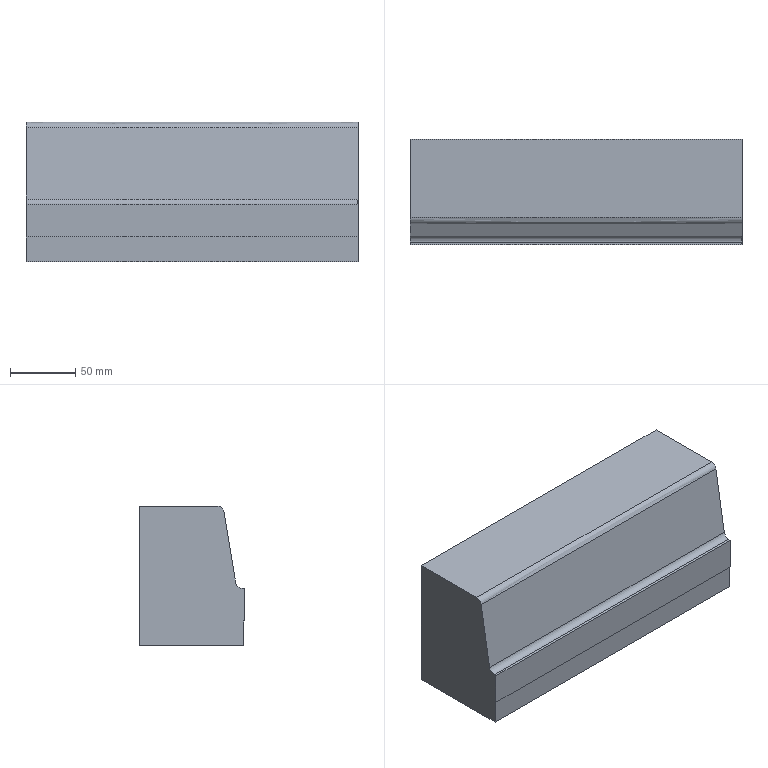Part | NX | features solid 2 | 1 solid | 22 faces | box 255 x 81.128 x 107.133 mm | volume 1996721 mm3 | plane 9 | cylinder 6 | spline 4 | cone 3 | commonest cylinder face diameters 12 x3 20 x2 10 x1
STEP:
#1=CARTESIAN_POINT('',(150.,175.,-20.));
#2=VERTEX_POINT('',#1);
#3=CARTESIAN_POINT('',(150.,175.,-30.));
#4=DIRECTION('',(0.,1.,0.));
#5=DIRECTION('',(0.,0.,1.));
#6=AXIS2_PLACEMENT_3D('',#3,#4,#5);
#7=CIRCLE('',#6,10.);
#8=EDGE_CURVE('',#2,#2,#7,.F.);
#9=ORIENTED_EDGE('',*,*,#8,.T.);
#10=EDGE_LOOP('',(#9));
#11=FACE_BOUND('',#10,.T.);
#12=CARTESIAN_POINT('',(-25.,175.,-20.));
#13=VERTEX_POINT('',#12);
#14=CARTESIAN_POINT('',(-25.,175.,-30.));
#15=DIRECTION('',(0.,1.,0.));
#16=DIRECTION('',(0.,0.,1.));
#17=AXIS2_PLACEMENT_3D('',#14,#15,#16);
#18=CIRCLE('',#17,10.);
#19=EDGE_CURVE('',#13,#13,#18,.F.);
#20=ORIENTED_EDGE('',*,*,#19,.T.);
#21=EDGE_LOOP('',(#20));
#22=FACE_BOUND('',#21,.T.);
#23=CARTESIAN_POINT('',(165.,175.,-11.));
#24=VERTEX_POINT('',#23);
#25=CARTESIAN_POINT('',(165.,175.,-5.));
#26=DIRECTION('',(0.,-1.,0.));
#27=DIRECTION('',(0.,0.,-1.));
#28=AXIS2_PLACEMENT_3D('',#25,#26,#27);
#29=CIRCLE('',#28,6.);
#30=EDGE_CURVE('',#24,#24,#29,.T.);
#31=ORIENTED_EDGE('',*,*,#30,.T.);
#32=EDGE_LOOP('',(#31));
#33=FACE_BOUND('',#32,.T.);
#34=CARTESIAN_POINT('',(65.,175.,-36.));
#35=VERTEX_POINT('',#34);
#36=CARTESIAN_POINT('',(65.,175.,-30.));
#37=DIRECTION('',(0.,-1.,0.));
#38=DIRECTION('',(0.,0.,-1.));
#39=AXIS2_PLACEMENT_3D('',#36,#37,#38);
#40=CIRCLE('',#39,6.);
#41=EDGE_CURVE('',#35,#35,#40,.T.);
#42=ORIENTED_EDGE('',*,*,#41,.T.);
#43=EDGE_LOOP('',(#42));
#44=FACE_BOUND('',#43,.T.);
#45=CARTESIAN_POINT('',(-40.,175.,-11.));
#46=VERTEX_POINT('',#45);
#47=CARTESIAN_POINT('',(-40.,175.,-5.));
#48=DIRECTION('',(0.,-1.,0.));
#49=DIRECTION('',(0.,0.,-1.));
#50=AXIS2_PLACEMENT_3D('',#47,#48,#49);
#51=CIRCLE('',#50,6.);
#52=EDGE_CURVE('',#46,#46,#51,.T.);
#53=ORIENTED_EDGE('',*,*,#52,.T.);
#54=EDGE_LOOP('',(#53));
#55=FACE_BOUND('',#54,.T.);
#56=CARTESIAN_POINT('',(190.,175.,57.133));
#57=VERTEX_POINT('',#56);
#58=CARTESIAN_POINT('',(190.,175.,-50.));
#59=VERTEX_POINT('',#58);
#60=CARTESIAN_POINT('',(190.,175.,-10.));
#61=DIRECTION('',(0.,0.,-1.));
#62=VECTOR('',#61,1000.);
#63=LINE('',#60,#62);
#64=EDGE_CURVE('',#57,#59,#63,.T.);
#65=ORIENTED_EDGE('',*,*,#64,.T.);
#66=CARTESIAN_POINT('',(-65.,175.,-50.));
#67=VERTEX_POINT('',#66);
#68=CARTESIAN_POINT('',(695.224,175.,-50.));
#69=DIRECTION('',(-1.,0.,0.));
#70=VECTOR('',#69,1000.);
#71=LINE('',#68,#70);
#72=EDGE_CURVE('',#59,#67,#71,.T.);
#73=ORIENTED_EDGE('',*,*,#72,.T.);
#74=CARTESIAN_POINT('',(-65.,175.,57.133));
#75=VERTEX_POINT('',#74);
#76=CARTESIAN_POINT('',(-65.,175.,-10.));
#77=DIRECTION('',(0.,0.,-1.));
#78=VECTOR('',#77,1000.);
#79=LINE('',#76,#78);
#80=EDGE_CURVE('',#67,#75,#79,.F.);
#81=ORIENTED_EDGE('',*,*,#80,.T.);
#82=CARTESIAN_POINT('',(750.,175.,57.133));
#83=DIRECTION('',(-1.,0.,0.));
#84=VECTOR('',#83,1000.);
#85=LINE('',#82,#84);
#86=EDGE_CURVE('',#57,#75,#85,.T.);
#87=ORIENTED_EDGE('',*,*,#86,.F.);
#88=EDGE_LOOP('',(#65,#73,#81,#87));
#89=FACE_BOUND('',#88,.T.);
#90=CARTESIAN_POINT('',(750.,175.,-10.));
#91=DIRECTION('',(0.,1.,0.));
#92=DIRECTION('',(0.,0.,1.));
#93=AXIS2_PLACEMENT_3D('',#90,#91,#92);
#94=PLANE('',#93);
#95=ADVANCED_FACE('',(#11,#22,#33,#44,#55,#89),#94,.T.);
#96=CARTESIAN_POINT('',(190.,109.917,52.95));
#97=VERTEX_POINT('',#96);
#98=CARTESIAN_POINT('',(-65.,109.917,52.95));
#99=VERTEX_POINT('',#98);
#100=CARTESIAN_POINT('',(190.,109.917,52.95));
#101=CARTESIAN_POINT('',(105.,109.917,52.95));
#102=CARTESIAN_POINT('',(20.,109.917,52.95));
#103=CARTESIAN_POINT('',(-65.,109.917,52.95));
#104=B_SPLINE_CURVE_WITH_KNOTS('',3,(#100,#101,#102,#103),.UNSPECIFIED.,.F.,.F.,(4,4),(0.1755,0.623),.UNSPECIFIED.);
#105=EDGE_CURVE('',#97,#99,#104,.T.);
#106=ORIENTED_EDGE('',*,*,#105,.F.);
#107=CARTESIAN_POINT('',(190.,114.85,57.133));
#108=VERTEX_POINT('',#107);
#109=CARTESIAN_POINT('',(190.,114.85,52.133));
#110=DIRECTION('',(1.,0.,0.));
#111=DIRECTION('',(0.,0.,-1.));
#112=AXIS2_PLACEMENT_3D('',#109,#110,#111);
#113=CIRCLE('',#112,5.);
#114=EDGE_CURVE('',#97,#108,#113,.F.);
#115=ORIENTED_EDGE('',*,*,#114,.T.);
#116=CARTESIAN_POINT('',(-65.,114.85,57.133));
#117=VERTEX_POINT('',#116);
#118=CARTESIAN_POINT('',(-65.,114.85,57.133));
#119=CARTESIAN_POINT('',(20.,114.85,57.133));
#120=CARTESIAN_POINT('',(105.,114.85,57.133));
#121=CARTESIAN_POINT('',(190.,114.85,57.133));
#122=B_SPLINE_CURVE_WITH_KNOTS('',3,(#118,#119,#120,#121),.UNSPECIFIED.,.F.,.F.,(4,4),(0.377,0.8245),.UNSPECIFIED.);
#123=EDGE_CURVE('',#117,#108,#122,.T.);
#124=ORIENTED_EDGE('',*,*,#123,.F.);
#125=CARTESIAN_POINT('',(-65.,114.85,52.133));
#126=DIRECTION('',(1.,0.,0.));
#127=DIRECTION('',(0.,0.,-1.));
#128=AXIS2_PLACEMENT_3D('',#125,#126,#127);
#129=CIRCLE('',#128,5.);
#130=EDGE_CURVE('',#99,#117,#129,.F.);
#131=ORIENTED_EDGE('',*,*,#130,.F.);
#132=EDGE_LOOP('',(#106,#115,#124,#131));
#133=FACE_BOUND('',#132,.T.);
#134=CARTESIAN_POINT('',(190.,114.85,57.133));
#135=CARTESIAN_POINT('',(190.,110.61,57.133));
#136=CARTESIAN_POINT('',(190.,109.917,52.95));
#137=CARTESIAN_POINT('',(105.,114.85,57.133));
#138=CARTESIAN_POINT('',(105.,110.61,57.133));
#139=CARTESIAN_POINT('',(105.,109.917,52.95));
#140=CARTESIAN_POINT('',(20.,114.85,57.133));
#141=CARTESIAN_POINT('',(20.,110.61,57.133));
#142=CARTESIAN_POINT('',(20.,109.917,52.95));
#143=CARTESIAN_POINT('',(-65.,114.85,57.133));
#144=CARTESIAN_POINT('',(-65.,110.61,57.133));
#145=CARTESIAN_POINT('',(-65.,109.917,52.95));
#146=(BOUNDED_SURFACE()B_SPLINE_SURFACE(3,2,((#134,#135,#136),(#137,#138,#139),(#140,#141,#142),(#143,#144,#145)),.UNSPECIFIED.,.F.,.F.,.F.)B_SPLINE_SURFACE_WITH_KNOTS((4,4),(3,3),(0.2812,0.5362),(0.,1.),.PIECEWISE_BEZIER_KNOTS.)GEOMETRIC_REPRESENTATION_ITEM()RATIONAL_B_SPLINE_SURFACE(((1.,0.7627,1.),(1.,0.7627,1.),(1.,0.7627,1.),(1.,0.7627,1.)))REPRESENTATION_ITEM('')SURFACE());
#147=ADVANCED_FACE('',(#133),#146,.T.);
#148=CARTESIAN_POINT('',(190.,100.848,-1.821));
#149=VERTEX_POINT('',#148);
#150=CARTESIAN_POINT('',(-65.,100.848,-1.821));
#151=VERTEX_POINT('',#150);
#152=CARTESIAN_POINT('',(190.,100.848,-1.821));
#153=CARTESIAN_POINT('',(105.,100.848,-1.821));
#154=CARTESIAN_POINT('',(20.,100.848,-1.821));
#155=CARTESIAN_POINT('',(-65.,100.848,-1.821));
#156=B_SPLINE_CURVE_WITH_KNOTS('',3,(#152,#153,#154,#155),.UNSPECIFIED.,.F.,.F.,(4,4),(0.1755,0.623),.UNSPECIFIED.);
#157=EDGE_CURVE('',#149,#151,#156,.T.);
#158=ORIENTED_EDGE('',*,*,#157,.F.);
#159=CARTESIAN_POINT('',(190.,105.878,28.559));
#160=DIRECTION('',(0.,0.1634,0.9866));
#161=VECTOR('',#160,1000.);
#162=LINE('',#159,#161);
#163=EDGE_CURVE('',#149,#97,#162,.T.);
#164=ORIENTED_EDGE('',*,*,#163,.T.);
#165=ORIENTED_EDGE('',*,*,#105,.T.);
#166=CARTESIAN_POINT('',(-65.,105.878,28.559));
#167=DIRECTION('',(0.,0.1634,0.9866));
#168=VECTOR('',#167,1000.);
#169=LINE('',#166,#168);
#170=EDGE_CURVE('',#151,#99,#169,.T.);
#171=ORIENTED_EDGE('',*,*,#170,.F.);
#172=EDGE_LOOP('',(#158,#164,#165,#171));
#173=FACE_BOUND('',#172,.T.);
#174=CARTESIAN_POINT('',(733.717,98.479,-16.126));
#175=CARTESIAN_POINT('',(-723.536,98.479,-16.126));
#176=CARTESIAN_POINT('',(733.717,113.278,73.243));
#177=CARTESIAN_POINT('',(-723.536,113.278,73.243));
#178=B_SPLINE_SURFACE_WITH_KNOTS('',1,1,((#174,#175),(#176,#177)),.PLANE_SURF.,.F.,.F.,.F.,(2,2),(2,2),(0.,1.902),(0.,1.),.UNSPECIFIED.);
#179=ADVANCED_FACE('',(#173),#178,.T.);
#180=CARTESIAN_POINT('',(190.,95.872,-6.004));
#181=VERTEX_POINT('',#180);
#182=CARTESIAN_POINT('',(190.,95.915,-1.004));
#183=DIRECTION('',(1.,0.,0.));
#184=DIRECTION('',(0.,0.,-1.));
#185=AXIS2_PLACEMENT_3D('',#182,#183,#184);
#186=CIRCLE('',#185,5.);
#187=EDGE_CURVE('',#149,#181,#186,.F.);
#188=ORIENTED_EDGE('',*,*,#187,.F.);
#189=ORIENTED_EDGE('',*,*,#157,.T.);
#190=CARTESIAN_POINT('',(-65.,95.872,-6.004));
#191=VERTEX_POINT('',#190);
#192=CARTESIAN_POINT('',(-65.,95.915,-1.004));
#193=DIRECTION('',(1.,0.,0.));
#194=DIRECTION('',(0.,0.,-1.));
#195=AXIS2_PLACEMENT_3D('',#192,#193,#194);
#196=CIRCLE('',#195,5.);
#197=EDGE_CURVE('',#151,#191,#196,.F.);
#198=ORIENTED_EDGE('',*,*,#197,.T.);
#199=CARTESIAN_POINT('',(-65.,95.872,-6.004));
#200=CARTESIAN_POINT('',(20.,95.872,-6.004));
#201=CARTESIAN_POINT('',(105.,95.872,-6.004));
#202=CARTESIAN_POINT('',(190.,95.872,-6.004));
#203=B_SPLINE_CURVE_WITH_KNOTS('',3,(#199,#200,#201,#202),.UNSPECIFIED.,.F.,.F.,(4,4),(0.377,0.8245),.UNSPECIFIED.);
#204=EDGE_CURVE('',#191,#181,#203,.T.);
#205=ORIENTED_EDGE('',*,*,#204,.T.);
#206=EDGE_LOOP('',(#188,#189,#198,#205));
#207=FACE_BOUND('',#206,.T.);
#208=CARTESIAN_POINT('',(6000290.,95.915,-1.004));
#209=DIRECTION('',(-1.,0.,0.));
#210=DIRECTION('',(0.,-0.1634,-0.9866));
#211=AXIS2_PLACEMENT_3D('',#208,#209,#210);
#212=CYLINDRICAL_SURFACE('',#211,5.);
#213=ADVANCED_FACE('',(#207),#212,.F.);
#214=CARTESIAN_POINT('',(190.,93.872,-5.987));
#215=VERTEX_POINT('',#214);
#216=CARTESIAN_POINT('',(190.,171.032,-6.646));
#217=DIRECTION('',(0.,-1.,0.008536));
#218=VECTOR('',#217,1000.);
#219=LINE('',#216,#218);
#220=EDGE_CURVE('',#181,#215,#219,.T.);
#221=ORIENTED_EDGE('',*,*,#220,.F.);
#222=ORIENTED_EDGE('',*,*,#204,.F.);
#223=CARTESIAN_POINT('',(-65.,93.872,-5.987));
#224=VERTEX_POINT('',#223);
#225=CARTESIAN_POINT('',(-65.,171.032,-6.646));
#226=DIRECTION('',(0.,-1.,0.008536));
#227=VECTOR('',#226,1000.);
#228=LINE('',#225,#227);
#229=EDGE_CURVE('',#191,#224,#228,.T.);
#230=ORIENTED_EDGE('',*,*,#229,.T.);
#231=CARTESIAN_POINT('',(290.,93.872,-5.987));
#232=DIRECTION('',(1.,0.,0.));
#233=VECTOR('',#232,1000.);
#234=LINE('',#231,#233);
#235=EDGE_CURVE('',#224,#215,#234,.T.);
#236=ORIENTED_EDGE('',*,*,#235,.T.);
#237=EDGE_LOOP('',(#221,#222,#230,#236));
#238=FACE_BOUND('',#237,.T.);
#239=CARTESIAN_POINT('',(120.529,171.032,-6.646));
#240=DIRECTION('',(0.,-0.008536,-1.));
#241=DIRECTION('',(0.,-1.,0.008536));
#242=AXIS2_PLACEMENT_3D('',#239,#240,#241);
#243=PLANE('',#242);
#244=ADVANCED_FACE('',(#238),#243,.F.);
#245=CARTESIAN_POINT('',(190.,93.872,-30.987));
#246=VERTEX_POINT('',#245);
#247=CARTESIAN_POINT('',(-65.,93.872,-30.987));
#248=VERTEX_POINT('',#247);
#249=CARTESIAN_POINT('',(190.,93.872,-30.987));
#250=CARTESIAN_POINT('',(105.,93.872,-30.987));
#251=CARTESIAN_POINT('',(20.,93.872,-30.987));
#252=CARTESIAN_POINT('',(-65.,93.872,-30.987));
#253=B_SPLINE_CURVE_WITH_KNOTS('',3,(#249,#250,#251,#252),.UNSPECIFIED.,.F.,.F.,(4,4),(0.1,0.355),.UNSPECIFIED.);
#254=EDGE_CURVE('',#246,#248,#253,.T.);
#255=ORIENTED_EDGE('',*,*,#254,.F.);
#256=CARTESIAN_POINT('',(190.,93.872,200.));
#257=DIRECTION('',(0.,0.,1.));
#258=VECTOR('',#257,1000.);
#259=LINE('',#256,#258);
#260=EDGE_CURVE('',#246,#215,#259,.T.);
#261=ORIENTED_EDGE('',*,*,#260,.T.);
#262=ORIENTED_EDGE('',*,*,#235,.F.);
#263=CARTESIAN_POINT('',(-65.,93.872,200.));
#264=DIRECTION('',(0.,0.,1.));
#265=VECTOR('',#264,1000.);
#266=LINE('',#263,#265);
#267=EDGE_CURVE('',#248,#224,#266,.T.);
#268=ORIENTED_EDGE('',*,*,#267,.F.);
#269=EDGE_LOOP('',(#255,#261,#262,#268));
#270=FACE_BOUND('',#269,.T.);
#271=CARTESIAN_POINT('',(290.,93.872,200.));
#272=DIRECTION('',(0.,-1.,0.));
#273=DIRECTION('',(1.,0.,0.));
#274=AXIS2_PLACEMENT_3D('',#271,#272,#273);
#275=PLANE('',#274);
#276=ADVANCED_FACE('',(#270),#275,.T.);
#277=CARTESIAN_POINT('',(-65.,94.872,-30.987));
#278=VERTEX_POINT('',#277);
#279=CARTESIAN_POINT('',(-65.,93.872,-30.987));
#280=CARTESIAN_POINT('',(-65.,94.206,-30.987));
#281=CARTESIAN_POINT('',(-65.,94.539,-30.987));
#282=CARTESIAN_POINT('',(-65.,94.872,-30.987));
#283=B_SPLINE_CURVE_WITH_KNOTS('',3,(#279,#280,#281,#282),.UNSPECIFIED.,.F.,.F.,(4,4),(0.0003492,0.001349),.UNSPECIFIED.);
#284=EDGE_CURVE('',#248,#278,#283,.T.);
#285=ORIENTED_EDGE('',*,*,#284,.T.);
#286=CARTESIAN_POINT('',(190.,94.889,-30.987));
#287=VERTEX_POINT('',#286);
#288=CARTESIAN_POINT('',(190.,94.889,-30.987));
#289=CARTESIAN_POINT('',(105.,94.866,-30.987));
#290=CARTESIAN_POINT('',(20.,94.872,-30.987));
#291=CARTESIAN_POINT('',(-65.,94.872,-30.987));
#292=B_SPLINE_CURVE_WITH_KNOTS('',3,(#288,#289,#290,#291),.UNSPECIFIED.,.F.,.F.,(4,4),(0.1333,0.3889),.UNSPECIFIED.);
#293=EDGE_CURVE('',#278,#287,#292,.F.);
#294=ORIENTED_EDGE('',*,*,#293,.T.);
#295=CARTESIAN_POINT('',(190.,93.872,-30.987));
#296=CARTESIAN_POINT('',(190.,94.211,-30.987));
#297=CARTESIAN_POINT('',(190.,94.55,-30.987));
#298=CARTESIAN_POINT('',(190.,94.889,-30.987));
#299=B_SPLINE_CURVE_WITH_KNOTS('',3,(#295,#296,#297,#298),.UNSPECIFIED.,.F.,.F.,(4,4),(0.0003325,0.001349),.UNSPECIFIED.);
#300=EDGE_CURVE('',#246,#287,#299,.T.);
#301=ORIENTED_EDGE('',*,*,#300,.F.);
#302=ORIENTED_EDGE('',*,*,#254,.T.);
#303=EDGE_LOOP('',(#285,#294,#301,#302));
#304=FACE_BOUND('',#303,.T.);
#305=CARTESIAN_POINT('',(-65.,94.872,-30.987));
#306=CARTESIAN_POINT('',(-41.607,94.872,-30.987));
#307=CARTESIAN_POINT('',(-18.213,94.872,-30.987));
#308=CARTESIAN_POINT('',(52.65,94.872,-30.987));
#309=CARTESIAN_POINT('',(100.12,94.872,-30.987));
#310=CARTESIAN_POINT('',(162.237,94.882,-30.987));
#311=CARTESIAN_POINT('',(176.884,94.885,-30.987));
#312=CARTESIAN_POINT('',(191.53,94.889,-30.987));
#313=CARTESIAN_POINT('',(-65.,93.849,-30.987));
#314=CARTESIAN_POINT('',(-41.607,93.849,-30.987));
#315=CARTESIAN_POINT('',(-18.213,93.849,-30.987));
#316=CARTESIAN_POINT('',(52.65,93.849,-30.987));
#317=CARTESIAN_POINT('',(100.12,93.849,-30.987));
#318=CARTESIAN_POINT('',(162.237,93.859,-30.987));
#319=CARTESIAN_POINT('',(176.884,93.863,-30.987));
#320=CARTESIAN_POINT('',(191.53,93.867,-30.987));
#321=B_SPLINE_SURFACE_WITH_KNOTS('',1,3,((#305,#306,#307,#308,#309,#310,#311,#312),(#313,#314,#315,#316,#317,#318,#319,#320)),.RULED_SURF.,.F.,.F.,.F.,(2,2),(4,2,2,4),(0.4,0.5023),(0.6129,0.6894,0.8447,0.8926),.UNSPECIFIED.);
#322=ADVANCED_FACE('',(#304),#321,.F.);
#323=ORIENTED_EDGE('',*,*,#293,.F.);
#324=CARTESIAN_POINT('',(-65.,94.872,-50.));
#325=VERTEX_POINT('',#324);
#326=CARTESIAN_POINT('',(-65.,94.872,-50.));
#327=DIRECTION('',(0.,0.,-1.));
#328=VECTOR('',#327,1000.);
#329=LINE('',#326,#328);
#330=EDGE_CURVE('',#325,#278,#329,.F.);
#331=ORIENTED_EDGE('',*,*,#330,.F.);
#332=CARTESIAN_POINT('',(190.,94.889,-50.));
#333=VERTEX_POINT('',#332);
#334=CARTESIAN_POINT('',(190.,94.889,-50.));
#335=CARTESIAN_POINT('',(105.,94.866,-50.));
#336=CARTESIAN_POINT('',(20.,94.872,-50.));
#337=CARTESIAN_POINT('',(-65.,94.872,-50.));
#338=B_SPLINE_CURVE_WITH_KNOTS('',3,(#334,#335,#336,#337),.UNSPECIFIED.,.F.,.F.,(4,4),(0.7975,1.053),.UNSPECIFIED.);
#339=EDGE_CURVE('',#333,#325,#338,.T.);
#340=ORIENTED_EDGE('',*,*,#339,.F.);
#341=CARTESIAN_POINT('',(190.,94.889,-40.494));
#342=DIRECTION('',(0.,0.,-1.));
#343=VECTOR('',#342,1000.);
#344=LINE('',#341,#343);
#345=EDGE_CURVE('',#287,#333,#344,.T.);
#346=ORIENTED_EDGE('',*,*,#345,.F.);
#347=EDGE_LOOP('',(#323,#331,#340,#346));
#348=FACE_BOUND('',#347,.T.);
#349=CARTESIAN_POINT('',(-65.,94.872,-30.987));
#350=CARTESIAN_POINT('',(-65.,94.872,-50.114));
#351=CARTESIAN_POINT('',(19.999,94.872,-30.987));
#352=CARTESIAN_POINT('',(19.999,94.872,-50.114));
#353=CARTESIAN_POINT('',(104.998,94.866,-30.987));
#354=CARTESIAN_POINT('',(104.998,94.866,-50.114));
#355=CARTESIAN_POINT('',(190.,94.889,-30.987));
#356=CARTESIAN_POINT('',(190.,94.889,-50.114));
#357=B_SPLINE_SURFACE_WITH_KNOTS('',3,1,((#349,#350),(#351,#352),(#353,#354),(#355,#356)),.SURF_OF_LINEAR_EXTRUSION.,.F.,.F.,.F.,(4,4),(2,2),(0.6129,0.891),(0.,1.),.PIECEWISE_BEZIER_KNOTS.);
#358=ADVANCED_FACE('',(#348),#357,.F.);
#359=ORIENTED_EDGE('',*,*,#300,.T.);
#360=ORIENTED_EDGE('',*,*,#345,.T.);
#361=CARTESIAN_POINT('',(190.,83.819,-50.));
#362=DIRECTION('',(0.,1.,0.));
#363=VECTOR('',#362,1000.);
#364=LINE('',#361,#363);
#365=EDGE_CURVE('',#333,#59,#364,.T.);
#366=ORIENTED_EDGE('',*,*,#365,.T.);
#367=ORIENTED_EDGE('',*,*,#64,.F.);
#368=CARTESIAN_POINT('',(190.,110.61,57.133));
#369=DIRECTION('',(0.,-1.,0.));
#370=VECTOR('',#369,1000.);
#371=LINE('',#368,#370);
#372=EDGE_CURVE('',#57,#108,#371,.T.);
#373=ORIENTED_EDGE('',*,*,#372,.T.);
#374=ORIENTED_EDGE('',*,*,#114,.F.);
#375=ORIENTED_EDGE('',*,*,#163,.F.);
#376=ORIENTED_EDGE('',*,*,#187,.T.);
#377=ORIENTED_EDGE('',*,*,#220,.T.);
#378=ORIENTED_EDGE('',*,*,#260,.F.);
#379=EDGE_LOOP('',(#359,#360,#366,#367,#373,#374,#375,#376,#377,#378));
#380=FACE_BOUND('',#379,.T.);
#381=CARTESIAN_POINT('',(190.,-360.,0.));
#382=DIRECTION('',(1.,0.,0.));
#383=DIRECTION('',(0.,0.,-1.));
#384=AXIS2_PLACEMENT_3D('',#381,#382,#383);
#385=PLANE('',#384);
#386=ADVANCED_FACE('',(#380),#385,.T.);
#387=ORIENTED_EDGE('',*,*,#372,.F.);
#388=ORIENTED_EDGE('',*,*,#86,.T.);
#389=CARTESIAN_POINT('',(-65.,110.61,57.133));
#390=DIRECTION('',(0.,-1.,0.));
#391=VECTOR('',#390,1000.);
#392=LINE('',#389,#391);
#393=EDGE_CURVE('',#75,#117,#392,.T.);
#394=ORIENTED_EDGE('',*,*,#393,.T.);
#395=ORIENTED_EDGE('',*,*,#123,.T.);
#396=EDGE_LOOP('',(#387,#388,#394,#395));
#397=FACE_BOUND('',#396,.T.);
#398=CARTESIAN_POINT('',(290.,110.61,57.133));
#399=DIRECTION('',(0.,0.,-1.));
#400=DIRECTION('',(-1.,0.,0.));
#401=AXIS2_PLACEMENT_3D('',#398,#399,#400);
#402=PLANE('',#401);
#403=ADVANCED_FACE('',(#397),#402,.F.);
#404=ORIENTED_EDGE('',*,*,#330,.T.);
#405=ORIENTED_EDGE('',*,*,#284,.F.);
#406=ORIENTED_EDGE('',*,*,#267,.T.);
#407=ORIENTED_EDGE('',*,*,#229,.F.);
#408=ORIENTED_EDGE('',*,*,#197,.F.);
#409=ORIENTED_EDGE('',*,*,#170,.T.);
#410=ORIENTED_EDGE('',*,*,#130,.T.);
#411=ORIENTED_EDGE('',*,*,#393,.F.);
#412=ORIENTED_EDGE('',*,*,#80,.F.);
#413=CARTESIAN_POINT('',(-65.,-360.,-50.));
#414=DIRECTION('',(0.,-1.,0.));
#415=VECTOR('',#414,1000.);
#416=LINE('',#413,#415);
#417=EDGE_CURVE('',#325,#67,#416,.F.);
#418=ORIENTED_EDGE('',*,*,#417,.F.);
#419=EDGE_LOOP('',(#404,#405,#406,#407,#408,#409,#410,#411,#412,#418));
#420=FACE_BOUND('',#419,.T.);
#421=CARTESIAN_POINT('',(-65.,-360.,0.));
#422=DIRECTION('',(1.,0.,0.));
#423=DIRECTION('',(0.,0.,-1.));
#424=AXIS2_PLACEMENT_3D('',#421,#422,#423);
#425=PLANE('',#424);
#426=ADVANCED_FACE('',(#420),#425,.F.);
#427=ORIENTED_EDGE('',*,*,#72,.F.);
#428=ORIENTED_EDGE('',*,*,#365,.F.);
#429=ORIENTED_EDGE('',*,*,#339,.T.);
#430=ORIENTED_EDGE('',*,*,#417,.T.);
#431=EDGE_LOOP('',(#427,#428,#429,#430));
#432=FACE_BOUND('',#431,.T.);
#433=CARTESIAN_POINT('',(695.224,83.819,-50.));
#434=DIRECTION('',(0.,0.,1.));
#435=DIRECTION('',(1.,0.,0.));
#436=AXIS2_PLACEMENT_3D('',#433,#434,#435);
#437=PLANE('',#436);
#438=ADVANCED_FACE('',(#432),#437,.F.);
#439=CARTESIAN_POINT('',(-40.,145.,-11.));
#440=VERTEX_POINT('',#439);
#441=CARTESIAN_POINT('',(-40.,145.,-5.));
#442=DIRECTION('',(0.,-1.,0.));
#443=DIRECTION('',(0.,0.,-1.));
#444=AXIS2_PLACEMENT_3D('',#441,#442,#443);
#445=CIRCLE('',#444,6.);
#446=EDGE_CURVE('',#440,#440,#445,.T.);
#447=ORIENTED_EDGE('',*,*,#446,.F.);
#448=EDGE_LOOP('',(#447));
#449=FACE_BOUND('',#448,.T.);
#450=CARTESIAN_POINT('',(-40.,141.395,-5.));
#451=VERTEX_POINT('',#450);
#452=VERTEX_LOOP('',#451);
#453=FACE_BOUND('',#452,.T.);
#454=CARTESIAN_POINT('',(-40.,145.,-5.));
#455=DIRECTION('',(0.,1.,0.));
#456=DIRECTION('',(0.,0.,1.));
#457=AXIS2_PLACEMENT_3D('',#454,#455,#456);
#458=CONICAL_SURFACE('',#457,6.,1.03);
#459=ADVANCED_FACE('',(#449,#453),#458,.F.);
#460=ORIENTED_EDGE('',*,*,#446,.T.);
#461=EDGE_LOOP('',(#460));
#462=FACE_BOUND('',#461,.T.);
#463=ORIENTED_EDGE('',*,*,#52,.F.);
#464=EDGE_LOOP('',(#463));
#465=FACE_BOUND('',#464,.T.);
#466=CARTESIAN_POINT('',(-40.,175.,-5.));
#467=DIRECTION('',(0.,-1.,0.));
#468=DIRECTION('',(0.,0.,-1.));
#469=AXIS2_PLACEMENT_3D('',#466,#467,#468);
#470=CYLINDRICAL_SURFACE('',#469,6.);
#471=ADVANCED_FACE('',(#462,#465),#470,.F.);
#472=CARTESIAN_POINT('',(65.,145.,-36.));
#473=VERTEX_POINT('',#472);
#474=CARTESIAN_POINT('',(65.,145.,-30.));
#475=DIRECTION('',(0.,-1.,0.));
#476=DIRECTION('',(0.,0.,-1.));
#477=AXIS2_PLACEMENT_3D('',#474,#475,#476);
#478=CIRCLE('',#477,6.);
#479=EDGE_CURVE('',#473,#473,#478,.T.);
#480=ORIENTED_EDGE('',*,*,#479,.F.);
#481=EDGE_LOOP('',(#480));
#482=FACE_BOUND('',#481,.T.);
#483=CARTESIAN_POINT('',(65.,141.395,-30.));
#484=VERTEX_POINT('',#483);
#485=VERTEX_LOOP('',#484);
#486=FACE_BOUND('',#485,.T.);
#487=CARTESIAN_POINT('',(65.,145.,-30.));
#488=DIRECTION('',(0.,1.,0.));
#489=DIRECTION('',(0.,0.,1.));
#490=AXIS2_PLACEMENT_3D('',#487,#488,#489);
#491=CONICAL_SURFACE('',#490,6.,1.03);
#492=ADVANCED_FACE('',(#482,#486),#491,.F.);
#493=ORIENTED_EDGE('',*,*,#479,.T.);
#494=EDGE_LOOP('',(#493));
#495=FACE_BOUND('',#494,.T.);
#496=ORIENTED_EDGE('',*,*,#41,.F.);
#497=EDGE_LOOP('',(#496));
#498=FACE_BOUND('',#497,.T.);
#499=CARTESIAN_POINT('',(65.,175.,-30.));
#500=DIRECTION('',(0.,-1.,0.));
#501=DIRECTION('',(0.,0.,-1.));
#502=AXIS2_PLACEMENT_3D('',#499,#500,#501);
#503=CYLINDRICAL_SURFACE('',#502,6.);
#504=ADVANCED_FACE('',(#495,#498),#503,.F.);
#505=CARTESIAN_POINT('',(165.,145.,-11.));
#506=VERTEX_POINT('',#505);
#507=CARTESIAN_POINT('',(165.,145.,-5.));
#508=DIRECTION('',(0.,-1.,0.));
#509=DIRECTION('',(0.,0.,-1.));
#510=AXIS2_PLACEMENT_3D('',#507,#508,#509);
#511=CIRCLE('',#510,6.);
#512=EDGE_CURVE('',#506,#506,#511,.T.);
#513=ORIENTED_EDGE('',*,*,#512,.F.);
#514=EDGE_LOOP('',(#513));
#515=FACE_BOUND('',#514,.T.);
#516=CARTESIAN_POINT('',(165.,141.395,-5.));
#517=VERTEX_POINT('',#516);
#518=VERTEX_LOOP('',#517);
#519=FACE_BOUND('',#518,.T.);
#520=CARTESIAN_POINT('',(165.,145.,-5.));
#521=DIRECTION('',(0.,1.,0.));
#522=DIRECTION('',(0.,0.,1.));
#523=AXIS2_PLACEMENT_3D('',#520,#521,#522);
#524=CONICAL_SURFACE('',#523,6.,1.03);
#525=ADVANCED_FACE('',(#515,#519),#524,.F.);
#526=ORIENTED_EDGE('',*,*,#512,.T.);
#527=EDGE_LOOP('',(#526));
#528=FACE_BOUND('',#527,.T.);
#529=ORIENTED_EDGE('',*,*,#30,.F.);
#530=EDGE_LOOP('',(#529));
#531=FACE_BOUND('',#530,.T.);
#532=CARTESIAN_POINT('',(165.,175.,-5.));
#533=DIRECTION('',(0.,-1.,0.));
#534=DIRECTION('',(0.,0.,-1.));
#535=AXIS2_PLACEMENT_3D('',#532,#533,#534);
#536=CYLINDRICAL_SURFACE('',#535,6.);
#537=ADVANCED_FACE('',(#528,#531),#536,.F.);
#538=CARTESIAN_POINT('',(-25.,145.,-40.));
#539=VERTEX_POINT('',#538);
#540=CARTESIAN_POINT('',(-25.,145.,-30.));
#541=DIRECTION('',(0.,-1.,0.));
#542=DIRECTION('',(0.,0.,-1.));
#543=AXIS2_PLACEMENT_3D('',#540,#541,#542);
#544=CIRCLE('',#543,10.);
#545=EDGE_CURVE('',#539,#539,#544,.T.);
#546=ORIENTED_EDGE('',*,*,#545,.T.);
#547=EDGE_LOOP('',(#546));
#548=FACE_BOUND('',#547,.T.);
#549=ORIENTED_EDGE('',*,*,#19,.F.);
#550=EDGE_LOOP('',(#549));
#551=FACE_BOUND('',#550,.T.);
#552=CARTESIAN_POINT('',(-25.,175.,-30.));
#553=DIRECTION('',(0.,-1.,0.));
#554=DIRECTION('',(0.,0.,-1.));
#555=AXIS2_PLACEMENT_3D('',#552,#553,#554);
#556=CYLINDRICAL_SURFACE('',#555,10.);
#557=ADVANCED_FACE('',(#548,#551),#556,.F.);
#558=ORIENTED_EDGE('',*,*,#545,.F.);
#559=EDGE_LOOP('',(#558));
#560=FACE_BOUND('',#559,.T.);
#561=CARTESIAN_POINT('',(-25.,145.,-30.));
#562=DIRECTION('',(0.,-1.,0.));
#563=DIRECTION('',(0.,0.,-1.));
#564=AXIS2_PLACEMENT_3D('',#561,#562,#563);
#565=PLANE('',#564);
#566=ADVANCED_FACE('',(#560),#565,.F.);
#567=CARTESIAN_POINT('',(150.,145.,-40.));
#568=VERTEX_POINT('',#567);
#569=CARTESIAN_POINT('',(150.,145.,-30.));
#570=DIRECTION('',(0.,-1.,0.));
#571=DIRECTION('',(0.,0.,-1.));
#572=AXIS2_PLACEMENT_3D('',#569,#570,#571);
#573=CIRCLE('',#572,10.);
#574=EDGE_CURVE('',#568,#568,#573,.T.);
#575=ORIENTED_EDGE('',*,*,#574,.T.);
#576=EDGE_LOOP('',(#575));
#577=FACE_BOUND('',#576,.T.);
#578=ORIENTED_EDGE('',*,*,#8,.F.);
#579=EDGE_LOOP('',(#578));
#580=FACE_BOUND('',#579,.T.);
#581=CARTESIAN_POINT('',(150.,175.,-30.));
#582=DIRECTION('',(0.,-1.,0.));
#583=DIRECTION('',(0.,0.,-1.));
#584=AXIS2_PLACEMENT_3D('',#581,#582,#583);
#585=CYLINDRICAL_SURFACE('',#584,10.);
#586=ADVANCED_FACE('',(#577,#580),#585,.F.);
#587=ORIENTED_EDGE('',*,*,#574,.F.);
#588=EDGE_LOOP('',(#587));
#589=FACE_BOUND('',#588,.T.);
#590=CARTESIAN_POINT('',(150.,145.,-30.));
#591=DIRECTION('',(0.,-1.,0.));
#592=DIRECTION('',(0.,0.,-1.));
#593=AXIS2_PLACEMENT_3D('',#590,#591,#592);
#594=PLANE('',#593);
#595=ADVANCED_FACE('',(#589),#594,.F.);
#596=CLOSED_SHELL('',(#95,#147,#179,#213,#244,#276,#322,#358,#386,#403,#426,#438,#459,#471,#492,#504,#525,#537,#557,#566,#586,#595));
#597=MANIFOLD_SOLID_BREP('',#596);
#598=(LENGTH_UNIT()NAMED_UNIT(*)SI_UNIT(.MILLI.,.METRE.));
#599=UNCERTAINTY_MEASURE_WITH_UNIT(LENGTH_MEASURE(0.0508),#598,'','');
#600=(NAMED_UNIT(*)PLANE_ANGLE_UNIT()SI_UNIT($,.RADIAN.));
#601=(NAMED_UNIT(*)SI_UNIT($,.STERADIAN.)SOLID_ANGLE_UNIT());
#602=(GEOMETRIC_REPRESENTATION_CONTEXT(3)GLOBAL_UNCERTAINTY_ASSIGNED_CONTEXT((#599))GLOBAL_UNIT_ASSIGNED_CONTEXT((#598,#600,#601))REPRESENTATION_CONTEXT('',''));
#603=ADVANCED_BREP_SHAPE_REPRESENTATION('',(#597),#602);